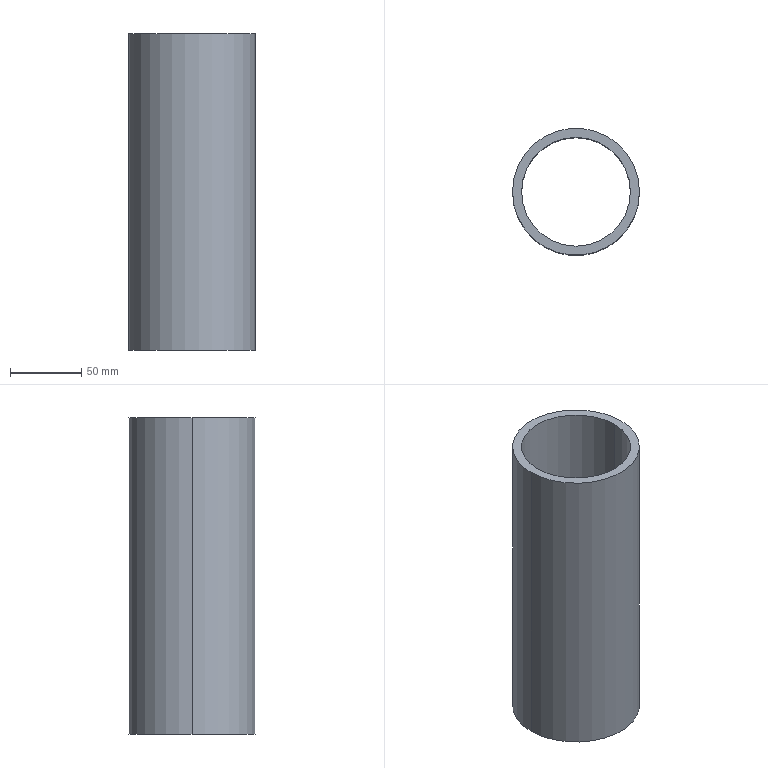Part | SolidWorks | features Extrusion 1 | 1 solid | 6 faces | box 88.9 x 88.9 x 222 mm | volume 365589 mm3 | cylinder 4 | plane 2 | commonest cylinder face diameters 76.2 x2 88.9 x2
STEP:
#1=CARTESIAN_POINT('',(-38.1,0.,111.));
#2=VERTEX_POINT('',#1);
#3=CARTESIAN_POINT('',(38.1,0.,111.));
#4=VERTEX_POINT('',#3);
#5=CARTESIAN_POINT('',(0.,0.,111.));
#6=DIRECTION('',(0.,0.,1.));
#7=DIRECTION('',(1.,0.,0.));
#8=AXIS2_PLACEMENT_3D('',#5,#6,#7);
#9=CIRCLE('',#8,38.1);
#10=EDGE_CURVE('',#2,#4,#9,.T.);
#11=ORIENTED_EDGE('',*,*,#10,.T.);
#12=CARTESIAN_POINT('',(38.1,0.,-111.));
#13=VERTEX_POINT('',#12);
#14=CARTESIAN_POINT('',(38.1,0.,111.));
#15=DIRECTION('',(0.,0.,-1.));
#16=VECTOR('',#15,1000.);
#17=LINE('',#14,#16);
#18=EDGE_CURVE('',#4,#13,#17,.T.);
#19=ORIENTED_EDGE('',*,*,#18,.T.);
#20=CARTESIAN_POINT('',(-38.1,0.,-111.));
#21=VERTEX_POINT('',#20);
#22=CARTESIAN_POINT('',(0.,0.,-111.));
#23=DIRECTION('',(0.,0.,1.));
#24=DIRECTION('',(1.,0.,0.));
#25=AXIS2_PLACEMENT_3D('',#22,#23,#24);
#26=CIRCLE('',#25,38.1);
#27=EDGE_CURVE('',#21,#13,#26,.T.);
#28=ORIENTED_EDGE('',*,*,#27,.F.);
#29=CARTESIAN_POINT('',(-38.1,0.,111.));
#30=DIRECTION('',(0.,0.,-1.));
#31=VECTOR('',#30,1000.);
#32=LINE('',#29,#31);
#33=EDGE_CURVE('',#2,#21,#32,.T.);
#34=ORIENTED_EDGE('',*,*,#33,.F.);
#35=EDGE_LOOP('',(#11,#19,#28,#34));
#36=FACE_OUTER_BOUND('',#35,.T.);
#37=CARTESIAN_POINT('',(0.,0.,111.));
#38=DIRECTION('',(0.,0.,-1.));
#39=DIRECTION('',(-1.,0.,0.));
#40=AXIS2_PLACEMENT_3D('',#37,#38,#39);
#41=CYLINDRICAL_SURFACE('',#40,38.1);
#42=ADVANCED_FACE('',(#36),#41,.F.);
#43=CARTESIAN_POINT('',(44.45,0.,111.));
#44=VERTEX_POINT('',#43);
#45=CARTESIAN_POINT('',(-44.45,0.,111.));
#46=VERTEX_POINT('',#45);
#47=CARTESIAN_POINT('',(0.,0.,111.));
#48=DIRECTION('',(0.,0.,1.));
#49=DIRECTION('',(1.,0.,0.));
#50=AXIS2_PLACEMENT_3D('',#47,#48,#49);
#51=CIRCLE('',#50,44.45);
#52=EDGE_CURVE('',#44,#46,#51,.T.);
#53=ORIENTED_EDGE('',*,*,#52,.F.);
#54=CARTESIAN_POINT('',(44.45,0.,-111.));
#55=VERTEX_POINT('',#54);
#56=CARTESIAN_POINT('',(44.45,0.,111.));
#57=DIRECTION('',(0.,0.,-1.));
#58=VECTOR('',#57,1000.);
#59=LINE('',#56,#58);
#60=EDGE_CURVE('',#44,#55,#59,.T.);
#61=ORIENTED_EDGE('',*,*,#60,.T.);
#62=CARTESIAN_POINT('',(-44.45,0.,-111.));
#63=VERTEX_POINT('',#62);
#64=CARTESIAN_POINT('',(0.,0.,-111.));
#65=DIRECTION('',(0.,0.,1.));
#66=DIRECTION('',(1.,0.,0.));
#67=AXIS2_PLACEMENT_3D('',#64,#65,#66);
#68=CIRCLE('',#67,44.45);
#69=EDGE_CURVE('',#55,#63,#68,.T.);
#70=ORIENTED_EDGE('',*,*,#69,.T.);
#71=CARTESIAN_POINT('',(-44.45,0.,111.));
#72=DIRECTION('',(0.,0.,-1.));
#73=VECTOR('',#72,1000.);
#74=LINE('',#71,#73);
#75=EDGE_CURVE('',#46,#63,#74,.T.);
#76=ORIENTED_EDGE('',*,*,#75,.F.);
#77=EDGE_LOOP('',(#53,#61,#70,#76));
#78=FACE_OUTER_BOUND('',#77,.T.);
#79=CARTESIAN_POINT('',(0.,0.,111.));
#80=DIRECTION('',(0.,0.,-1.));
#81=DIRECTION('',(-1.,0.,0.));
#82=AXIS2_PLACEMENT_3D('',#79,#80,#81);
#83=CYLINDRICAL_SURFACE('',#82,44.45);
#84=ADVANCED_FACE('',(#78),#83,.T.);
#85=CARTESIAN_POINT('',(0.,0.,111.));
#86=DIRECTION('',(0.,0.,1.));
#87=DIRECTION('',(1.,0.,0.));
#88=AXIS2_PLACEMENT_3D('',#85,#86,#87);
#89=CIRCLE('',#88,44.45);
#90=EDGE_CURVE('',#46,#44,#89,.T.);
#91=ORIENTED_EDGE('',*,*,#90,.T.);
#92=ORIENTED_EDGE('',*,*,#52,.T.);
#93=EDGE_LOOP('',(#91,#92));
#94=FACE_OUTER_BOUND('',#93,.T.);
#95=ORIENTED_EDGE('',*,*,#10,.F.);
#96=CARTESIAN_POINT('',(0.,0.,111.));
#97=DIRECTION('',(0.,0.,1.));
#98=DIRECTION('',(1.,0.,0.));
#99=AXIS2_PLACEMENT_3D('',#96,#97,#98);
#100=CIRCLE('',#99,38.1);
#101=EDGE_CURVE('',#4,#2,#100,.T.);
#102=ORIENTED_EDGE('',*,*,#101,.F.);
#103=EDGE_LOOP('',(#95,#102));
#104=FACE_BOUND('',#103,.T.);
#105=CARTESIAN_POINT('',(0.,0.,111.));
#106=DIRECTION('',(0.,0.,1.));
#107=DIRECTION('',(1.,0.,0.));
#108=AXIS2_PLACEMENT_3D('',#105,#106,#107);
#109=PLANE('',#108);
#110=ADVANCED_FACE('',(#94,#104),#109,.T.);
#111=CARTESIAN_POINT('',(0.,0.,-111.));
#112=DIRECTION('',(0.,0.,1.));
#113=DIRECTION('',(1.,0.,0.));
#114=AXIS2_PLACEMENT_3D('',#111,#112,#113);
#115=CIRCLE('',#114,44.45);
#116=EDGE_CURVE('',#63,#55,#115,.T.);
#117=ORIENTED_EDGE('',*,*,#116,.F.);
#118=ORIENTED_EDGE('',*,*,#69,.F.);
#119=EDGE_LOOP('',(#117,#118));
#120=FACE_OUTER_BOUND('',#119,.T.);
#121=ORIENTED_EDGE('',*,*,#27,.T.);
#122=CARTESIAN_POINT('',(0.,0.,-111.));
#123=DIRECTION('',(0.,0.,1.));
#124=DIRECTION('',(1.,0.,0.));
#125=AXIS2_PLACEMENT_3D('',#122,#123,#124);
#126=CIRCLE('',#125,38.1);
#127=EDGE_CURVE('',#13,#21,#126,.T.);
#128=ORIENTED_EDGE('',*,*,#127,.T.);
#129=EDGE_LOOP('',(#121,#128));
#130=FACE_BOUND('',#129,.T.);
#131=CARTESIAN_POINT('',(0.,0.,-111.));
#132=DIRECTION('',(0.,0.,1.));
#133=DIRECTION('',(1.,0.,0.));
#134=AXIS2_PLACEMENT_3D('',#131,#132,#133);
#135=PLANE('',#134);
#136=ADVANCED_FACE('',(#120,#130),#135,.F.);
#137=ORIENTED_EDGE('',*,*,#60,.F.);
#138=ORIENTED_EDGE('',*,*,#90,.F.);
#139=ORIENTED_EDGE('',*,*,#75,.T.);
#140=ORIENTED_EDGE('',*,*,#116,.T.);
#141=EDGE_LOOP('',(#137,#138,#139,#140));
#142=FACE_OUTER_BOUND('',#141,.T.);
#143=CARTESIAN_POINT('',(0.,0.,111.));
#144=DIRECTION('',(0.,0.,-1.));
#145=DIRECTION('',(-1.,0.,0.));
#146=AXIS2_PLACEMENT_3D('',#143,#144,#145);
#147=CYLINDRICAL_SURFACE('',#146,44.45);
#148=ADVANCED_FACE('',(#142),#147,.T.);
#149=ORIENTED_EDGE('',*,*,#18,.F.);
#150=ORIENTED_EDGE('',*,*,#101,.T.);
#151=ORIENTED_EDGE('',*,*,#33,.T.);
#152=ORIENTED_EDGE('',*,*,#127,.F.);
#153=EDGE_LOOP('',(#149,#150,#151,#152));
#154=FACE_OUTER_BOUND('',#153,.T.);
#155=CARTESIAN_POINT('',(0.,0.,111.));
#156=DIRECTION('',(0.,0.,-1.));
#157=DIRECTION('',(-1.,0.,0.));
#158=AXIS2_PLACEMENT_3D('',#155,#156,#157);
#159=CYLINDRICAL_SURFACE('',#158,38.1);
#160=ADVANCED_FACE('',(#154),#159,.F.);
#161=CLOSED_SHELL('',(#42,#84,#110,#136,#148,#160));
#162=MANIFOLD_SOLID_BREP('',#161);
#163=CARTESIAN_POINT('',(0.,0.,0.));
#164=DIRECTION('',(0.,0.,1.));
#165=DIRECTION('',(1.,0.,0.));
#166=AXIS2_PLACEMENT_3D('',#163,#164,#165);
#167=(LENGTH_UNIT()NAMED_UNIT(*)SI_UNIT(.MILLI.,.METRE.));
#168=UNCERTAINTY_MEASURE_WITH_UNIT(LENGTH_MEASURE(0.00001),#167,'','');
#169=(NAMED_UNIT(*)PLANE_ANGLE_UNIT()SI_UNIT($,.RADIAN.));
#170=(NAMED_UNIT(*)SI_UNIT($,.STERADIAN.)SOLID_ANGLE_UNIT());
#171=(GEOMETRIC_REPRESENTATION_CONTEXT(3)GLOBAL_UNCERTAINTY_ASSIGNED_CONTEXT((#168))GLOBAL_UNIT_ASSIGNED_CONTEXT((#167,#169,#170))REPRESENTATION_CONTEXT('',''));
#172=ADVANCED_BREP_SHAPE_REPRESENTATION('',(#162,#166),#171);